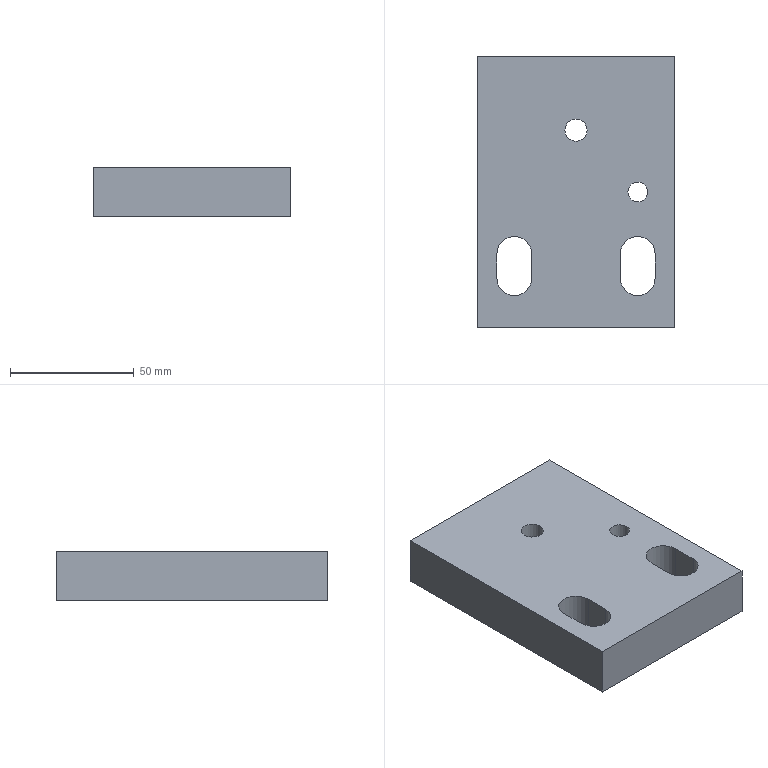Part | NX | features solid 2 | 1 solid | 18 faces | box 80 x 110 x 20 mm | volume 161289 mm3 | plane 11 | cylinder 7 | commonest cylinder face diameters 14 x4 8 x1 9 x1 13.5 x1
STEP:
#1=CARTESIAN_POINT('',(-1580.,335.,-55.));
#2=VERTEX_POINT('',#1);
#3=CARTESIAN_POINT('',(-1580.,445.,-55.));
#4=VERTEX_POINT('',#3);
#5=CARTESIAN_POINT('',(-1580.,375.,-55.));
#6=DIRECTION('',(0.,1.,0.));
#7=VECTOR('',#6,1000.);
#8=LINE('',#5,#7);
#9=EDGE_CURVE('',#2,#4,#8,.T.);
#10=ORIENTED_EDGE('',*,*,#9,.T.);
#11=CARTESIAN_POINT('',(-1500.,445.,-55.));
#12=VERTEX_POINT('',#11);
#13=CARTESIAN_POINT('',(-1580.,445.,-55.));
#14=DIRECTION('',(1.,0.,0.));
#15=VECTOR('',#14,1000.);
#16=LINE('',#13,#15);
#17=EDGE_CURVE('',#4,#12,#16,.T.);
#18=ORIENTED_EDGE('',*,*,#17,.T.);
#19=CARTESIAN_POINT('',(-1500.,335.,-55.));
#20=VERTEX_POINT('',#19);
#21=CARTESIAN_POINT('',(-1500.,475.,-55.));
#22=DIRECTION('',(0.,-1.,0.));
#23=VECTOR('',#22,1000.);
#24=LINE('',#21,#23);
#25=EDGE_CURVE('',#12,#20,#24,.T.);
#26=ORIENTED_EDGE('',*,*,#25,.T.);
#27=CARTESIAN_POINT('',(-1500.,335.,-55.));
#28=DIRECTION('',(-1.,0.,0.));
#29=VECTOR('',#28,1000.);
#30=LINE('',#27,#29);
#31=EDGE_CURVE('',#20,#2,#30,.T.);
#32=ORIENTED_EDGE('',*,*,#31,.T.);
#33=EDGE_LOOP('',(#10,#18,#26,#32));
#34=FACE_BOUND('',#33,.T.);
#35=CARTESIAN_POINT('',(-1572.,355.,-55.));
#36=VERTEX_POINT('',#35);
#37=CARTESIAN_POINT('',(-1572.,365.,-55.));
#38=VERTEX_POINT('',#37);
#39=CARTESIAN_POINT('',(-1572.,355.,-55.));
#40=DIRECTION('',(0.,1.,0.));
#41=VECTOR('',#40,1000.);
#42=LINE('',#39,#41);
#43=EDGE_CURVE('',#36,#38,#42,.T.);
#44=ORIENTED_EDGE('',*,*,#43,.F.);
#45=CARTESIAN_POINT('',(-1558.,355.,-55.));
#46=VERTEX_POINT('',#45);
#47=CARTESIAN_POINT('',(-1565.,355.,-55.));
#48=DIRECTION('',(0.,0.,1.));
#49=DIRECTION('',(1.,0.,0.));
#50=AXIS2_PLACEMENT_3D('',#47,#48,#49);
#51=CIRCLE('',#50,7.);
#52=EDGE_CURVE('',#36,#46,#51,.T.);
#53=ORIENTED_EDGE('',*,*,#52,.T.);
#54=CARTESIAN_POINT('',(-1558.,365.,-55.));
#55=VERTEX_POINT('',#54);
#56=CARTESIAN_POINT('',(-1558.,355.,-55.));
#57=DIRECTION('',(0.,1.,0.));
#58=VECTOR('',#57,1000.);
#59=LINE('',#56,#58);
#60=EDGE_CURVE('',#46,#55,#59,.T.);
#61=ORIENTED_EDGE('',*,*,#60,.T.);
#62=CARTESIAN_POINT('',(-1565.,365.,-55.));
#63=DIRECTION('',(0.,0.,1.));
#64=DIRECTION('',(1.,0.,0.));
#65=AXIS2_PLACEMENT_3D('',#62,#63,#64);
#66=CIRCLE('',#65,7.);
#67=EDGE_CURVE('',#55,#38,#66,.T.);
#68=ORIENTED_EDGE('',*,*,#67,.T.);
#69=EDGE_LOOP('',(#44,#53,#61,#68));
#70=FACE_BOUND('',#69,.T.);
#71=CARTESIAN_POINT('',(-1522.,355.,-55.));
#72=VERTEX_POINT('',#71);
#73=CARTESIAN_POINT('',(-1522.,365.,-55.));
#74=VERTEX_POINT('',#73);
#75=CARTESIAN_POINT('',(-1522.,355.,-55.));
#76=DIRECTION('',(0.,1.,0.));
#77=VECTOR('',#76,1000.);
#78=LINE('',#75,#77);
#79=EDGE_CURVE('',#72,#74,#78,.T.);
#80=ORIENTED_EDGE('',*,*,#79,.F.);
#81=CARTESIAN_POINT('',(-1508.,355.,-55.));
#82=VERTEX_POINT('',#81);
#83=CARTESIAN_POINT('',(-1515.,355.,-55.));
#84=DIRECTION('',(0.,0.,1.));
#85=DIRECTION('',(1.,0.,0.));
#86=AXIS2_PLACEMENT_3D('',#83,#84,#85);
#87=CIRCLE('',#86,7.);
#88=EDGE_CURVE('',#72,#82,#87,.T.);
#89=ORIENTED_EDGE('',*,*,#88,.T.);
#90=CARTESIAN_POINT('',(-1508.,365.,-55.));
#91=VERTEX_POINT('',#90);
#92=CARTESIAN_POINT('',(-1508.,355.,-55.));
#93=DIRECTION('',(0.,1.,0.));
#94=VECTOR('',#93,1000.);
#95=LINE('',#92,#94);
#96=EDGE_CURVE('',#82,#91,#95,.T.);
#97=ORIENTED_EDGE('',*,*,#96,.T.);
#98=CARTESIAN_POINT('',(-1515.,365.,-55.));
#99=DIRECTION('',(0.,0.,1.));
#100=DIRECTION('',(1.,0.,0.));
#101=AXIS2_PLACEMENT_3D('',#98,#99,#100);
#102=CIRCLE('',#101,7.);
#103=EDGE_CURVE('',#91,#74,#102,.T.);
#104=ORIENTED_EDGE('',*,*,#103,.T.);
#105=EDGE_LOOP('',(#80,#89,#97,#104));
#106=FACE_BOUND('',#105,.T.);
#107=CARTESIAN_POINT('',(-1533.25,415.,-55.));
#108=VERTEX_POINT('',#107);
#109=CARTESIAN_POINT('',(-1540.,415.,-55.));
#110=DIRECTION('',(0.,0.,1.));
#111=DIRECTION('',(1.,0.,0.));
#112=AXIS2_PLACEMENT_3D('',#109,#110,#111);
#113=CIRCLE('',#112,6.75);
#114=EDGE_CURVE('',#108,#108,#113,.T.);
#115=ORIENTED_EDGE('',*,*,#114,.T.);
#116=EDGE_LOOP('',(#115));
#117=FACE_BOUND('',#116,.T.);
#118=CARTESIAN_POINT('',(-1519.,390.,-55.));
#119=VERTEX_POINT('',#118);
#120=CARTESIAN_POINT('',(-1515.,390.,-55.));
#121=DIRECTION('',(0.,0.,-1.));
#122=DIRECTION('',(-1.,0.,0.));
#123=AXIS2_PLACEMENT_3D('',#120,#121,#122);
#124=CIRCLE('',#123,4.);
#125=EDGE_CURVE('',#119,#119,#124,.F.);
#126=ORIENTED_EDGE('',*,*,#125,.T.);
#127=EDGE_LOOP('',(#126));
#128=FACE_BOUND('',#127,.T.);
#129=CARTESIAN_POINT('',(-1580.,475.,-55.));
#130=DIRECTION('',(0.,0.,-1.));
#131=DIRECTION('',(-1.,0.,0.));
#132=AXIS2_PLACEMENT_3D('',#129,#130,#131);
#133=PLANE('',#132);
#134=ADVANCED_FACE('',(#34,#70,#106,#117,#128),#133,.T.);
#135=CARTESIAN_POINT('',(-1580.,335.,-35.));
#136=VERTEX_POINT('',#135);
#137=CARTESIAN_POINT('',(-1580.,445.,-35.));
#138=VERTEX_POINT('',#137);
#139=CARTESIAN_POINT('',(-1580.,375.,-35.));
#140=DIRECTION('',(0.,1.,0.));
#141=VECTOR('',#140,1000.);
#142=LINE('',#139,#141);
#143=EDGE_CURVE('',#136,#138,#142,.T.);
#144=ORIENTED_EDGE('',*,*,#143,.T.);
#145=CARTESIAN_POINT('',(-1580.,445.,-55.));
#146=DIRECTION('',(0.,0.,1.));
#147=VECTOR('',#146,1000.);
#148=LINE('',#145,#147);
#149=EDGE_CURVE('',#4,#138,#148,.T.);
#150=ORIENTED_EDGE('',*,*,#149,.F.);
#151=ORIENTED_EDGE('',*,*,#9,.F.);
#152=CARTESIAN_POINT('',(-1580.,335.,-55.));
#153=DIRECTION('',(0.,0.,1.));
#154=VECTOR('',#153,1000.);
#155=LINE('',#152,#154);
#156=EDGE_CURVE('',#2,#136,#155,.T.);
#157=ORIENTED_EDGE('',*,*,#156,.T.);
#158=EDGE_LOOP('',(#144,#150,#151,#157));
#159=FACE_BOUND('',#158,.T.);
#160=CARTESIAN_POINT('',(-1580.,375.,-55.));
#161=DIRECTION('',(1.,0.,0.));
#162=DIRECTION('',(0.,1.,0.));
#163=AXIS2_PLACEMENT_3D('',#160,#161,#162);
#164=PLANE('',#163);
#165=ADVANCED_FACE('',(#159),#164,.F.);
#166=CARTESIAN_POINT('',(-1500.,445.,-35.));
#167=VERTEX_POINT('',#166);
#168=CARTESIAN_POINT('',(-1580.,445.,-35.));
#169=DIRECTION('',(1.,0.,0.));
#170=VECTOR('',#169,1000.);
#171=LINE('',#168,#170);
#172=EDGE_CURVE('',#138,#167,#171,.T.);
#173=ORIENTED_EDGE('',*,*,#172,.T.);
#174=CARTESIAN_POINT('',(-1500.,445.,-55.));
#175=DIRECTION('',(0.,0.,1.));
#176=VECTOR('',#175,1000.);
#177=LINE('',#174,#176);
#178=EDGE_CURVE('',#12,#167,#177,.T.);
#179=ORIENTED_EDGE('',*,*,#178,.F.);
#180=ORIENTED_EDGE('',*,*,#17,.F.);
#181=ORIENTED_EDGE('',*,*,#149,.T.);
#182=EDGE_LOOP('',(#173,#179,#180,#181));
#183=FACE_BOUND('',#182,.T.);
#184=CARTESIAN_POINT('',(-1580.,445.,-55.));
#185=DIRECTION('',(0.,-1.,0.));
#186=DIRECTION('',(1.,0.,0.));
#187=AXIS2_PLACEMENT_3D('',#184,#185,#186);
#188=PLANE('',#187);
#189=ADVANCED_FACE('',(#183),#188,.F.);
#190=CARTESIAN_POINT('',(-1500.,335.,-35.));
#191=VERTEX_POINT('',#190);
#192=CARTESIAN_POINT('',(-1500.,475.,-35.));
#193=DIRECTION('',(0.,-1.,0.));
#194=VECTOR('',#193,1000.);
#195=LINE('',#192,#194);
#196=EDGE_CURVE('',#167,#191,#195,.T.);
#197=ORIENTED_EDGE('',*,*,#196,.T.);
#198=CARTESIAN_POINT('',(-1500.,335.,-55.));
#199=DIRECTION('',(0.,0.,1.));
#200=VECTOR('',#199,1000.);
#201=LINE('',#198,#200);
#202=EDGE_CURVE('',#20,#191,#201,.T.);
#203=ORIENTED_EDGE('',*,*,#202,.F.);
#204=ORIENTED_EDGE('',*,*,#25,.F.);
#205=ORIENTED_EDGE('',*,*,#178,.T.);
#206=EDGE_LOOP('',(#197,#203,#204,#205));
#207=FACE_BOUND('',#206,.T.);
#208=CARTESIAN_POINT('',(-1500.,475.,-55.));
#209=DIRECTION('',(-1.,0.,0.));
#210=DIRECTION('',(0.,0.,1.));
#211=AXIS2_PLACEMENT_3D('',#208,#209,#210);
#212=PLANE('',#211);
#213=ADVANCED_FACE('',(#207),#212,.F.);
#214=CARTESIAN_POINT('',(-1500.,335.,-35.));
#215=DIRECTION('',(-1.,0.,0.));
#216=VECTOR('',#215,1000.);
#217=LINE('',#214,#216);
#218=EDGE_CURVE('',#191,#136,#217,.T.);
#219=ORIENTED_EDGE('',*,*,#218,.T.);
#220=ORIENTED_EDGE('',*,*,#156,.F.);
#221=ORIENTED_EDGE('',*,*,#31,.F.);
#222=ORIENTED_EDGE('',*,*,#202,.T.);
#223=EDGE_LOOP('',(#219,#220,#221,#222));
#224=FACE_BOUND('',#223,.T.);
#225=CARTESIAN_POINT('',(-1500.,335.,-55.));
#226=DIRECTION('',(0.,1.,0.));
#227=DIRECTION('',(-1.,0.,0.));
#228=AXIS2_PLACEMENT_3D('',#225,#226,#227);
#229=PLANE('',#228);
#230=ADVANCED_FACE('',(#224),#229,.F.);
#231=CARTESIAN_POINT('',(-1519.,390.,-35.));
#232=VERTEX_POINT('',#231);
#233=CARTESIAN_POINT('',(-1515.,390.,-35.));
#234=DIRECTION('',(0.,0.,-1.));
#235=DIRECTION('',(-1.,0.,0.));
#236=AXIS2_PLACEMENT_3D('',#233,#234,#235);
#237=CIRCLE('',#236,4.);
#238=EDGE_CURVE('',#232,#232,#237,.T.);
#239=ORIENTED_EDGE('',*,*,#238,.T.);
#240=EDGE_LOOP('',(#239));
#241=FACE_BOUND('',#240,.T.);
#242=CARTESIAN_POINT('',(-1522.,355.,-35.));
#243=VERTEX_POINT('',#242);
#244=CARTESIAN_POINT('',(-1508.,355.,-35.));
#245=VERTEX_POINT('',#244);
#246=CARTESIAN_POINT('',(-1515.,355.,-35.));
#247=DIRECTION('',(0.,0.,1.));
#248=DIRECTION('',(1.,0.,0.));
#249=AXIS2_PLACEMENT_3D('',#246,#247,#248);
#250=CIRCLE('',#249,7.);
#251=EDGE_CURVE('',#243,#245,#250,.T.);
#252=ORIENTED_EDGE('',*,*,#251,.F.);
#253=CARTESIAN_POINT('',(-1522.,365.,-35.));
#254=VERTEX_POINT('',#253);
#255=CARTESIAN_POINT('',(-1522.,360.,-35.));
#256=DIRECTION('',(0.,1.,0.));
#257=VECTOR('',#256,1000.);
#258=LINE('',#255,#257);
#259=EDGE_CURVE('',#243,#254,#258,.T.);
#260=ORIENTED_EDGE('',*,*,#259,.T.);
#261=CARTESIAN_POINT('',(-1508.,365.,-35.));
#262=VERTEX_POINT('',#261);
#263=CARTESIAN_POINT('',(-1515.,365.,-35.));
#264=DIRECTION('',(0.,0.,1.));
#265=DIRECTION('',(1.,0.,0.));
#266=AXIS2_PLACEMENT_3D('',#263,#264,#265);
#267=CIRCLE('',#266,7.);
#268=EDGE_CURVE('',#262,#254,#267,.T.);
#269=ORIENTED_EDGE('',*,*,#268,.F.);
#270=CARTESIAN_POINT('',(-1508.,360.,-35.));
#271=DIRECTION('',(0.,1.,0.));
#272=VECTOR('',#271,1000.);
#273=LINE('',#270,#272);
#274=EDGE_CURVE('',#245,#262,#273,.T.);
#275=ORIENTED_EDGE('',*,*,#274,.F.);
#276=EDGE_LOOP('',(#252,#260,#269,#275));
#277=FACE_BOUND('',#276,.T.);
#278=CARTESIAN_POINT('',(-1572.,355.,-35.));
#279=VERTEX_POINT('',#278);
#280=CARTESIAN_POINT('',(-1558.,355.,-35.));
#281=VERTEX_POINT('',#280);
#282=CARTESIAN_POINT('',(-1565.,355.,-35.));
#283=DIRECTION('',(0.,0.,1.));
#284=DIRECTION('',(1.,0.,0.));
#285=AXIS2_PLACEMENT_3D('',#282,#283,#284);
#286=CIRCLE('',#285,7.);
#287=EDGE_CURVE('',#279,#281,#286,.T.);
#288=ORIENTED_EDGE('',*,*,#287,.F.);
#289=CARTESIAN_POINT('',(-1572.,365.,-35.));
#290=VERTEX_POINT('',#289);
#291=CARTESIAN_POINT('',(-1572.,360.,-35.));
#292=DIRECTION('',(0.,1.,0.));
#293=VECTOR('',#292,1000.);
#294=LINE('',#291,#293);
#295=EDGE_CURVE('',#279,#290,#294,.T.);
#296=ORIENTED_EDGE('',*,*,#295,.T.);
#297=CARTESIAN_POINT('',(-1558.,365.,-35.));
#298=VERTEX_POINT('',#297);
#299=CARTESIAN_POINT('',(-1565.,365.,-35.));
#300=DIRECTION('',(0.,0.,1.));
#301=DIRECTION('',(1.,0.,0.));
#302=AXIS2_PLACEMENT_3D('',#299,#300,#301);
#303=CIRCLE('',#302,7.);
#304=EDGE_CURVE('',#298,#290,#303,.T.);
#305=ORIENTED_EDGE('',*,*,#304,.F.);
#306=CARTESIAN_POINT('',(-1558.,360.,-35.));
#307=DIRECTION('',(0.,1.,0.));
#308=VECTOR('',#307,1000.);
#309=LINE('',#306,#308);
#310=EDGE_CURVE('',#281,#298,#309,.T.);
#311=ORIENTED_EDGE('',*,*,#310,.F.);
#312=EDGE_LOOP('',(#288,#296,#305,#311));
#313=FACE_BOUND('',#312,.T.);
#314=ORIENTED_EDGE('',*,*,#143,.F.);
#315=ORIENTED_EDGE('',*,*,#218,.F.);
#316=ORIENTED_EDGE('',*,*,#196,.F.);
#317=ORIENTED_EDGE('',*,*,#172,.F.);
#318=EDGE_LOOP('',(#314,#315,#316,#317));
#319=FACE_BOUND('',#318,.T.);
#320=CARTESIAN_POINT('',(-1544.5,415.,-35.));
#321=VERTEX_POINT('',#320);
#322=CARTESIAN_POINT('',(-1540.,415.,-35.));
#323=DIRECTION('',(0.,0.,-1.));
#324=DIRECTION('',(-1.,0.,0.));
#325=AXIS2_PLACEMENT_3D('',#322,#323,#324);
#326=CIRCLE('',#325,4.5);
#327=EDGE_CURVE('',#321,#321,#326,.F.);
#328=ORIENTED_EDGE('',*,*,#327,.F.);
#329=EDGE_LOOP('',(#328));
#330=FACE_BOUND('',#329,.T.);
#331=CARTESIAN_POINT('',(-1580.,475.,-35.));
#332=DIRECTION('',(0.,0.,-1.));
#333=DIRECTION('',(-1.,0.,0.));
#334=AXIS2_PLACEMENT_3D('',#331,#332,#333);
#335=PLANE('',#334);
#336=ADVANCED_FACE('',(#241,#277,#313,#319,#330),#335,.F.);
#337=ORIENTED_EDGE('',*,*,#295,.F.);
#338=CARTESIAN_POINT('',(-1572.,355.,-35.));
#339=DIRECTION('',(0.,0.,1.));
#340=VECTOR('',#339,1000.);
#341=LINE('',#338,#340);
#342=EDGE_CURVE('',#36,#279,#341,.T.);
#343=ORIENTED_EDGE('',*,*,#342,.F.);
#344=ORIENTED_EDGE('',*,*,#43,.T.);
#345=CARTESIAN_POINT('',(-1572.,365.,-35.));
#346=DIRECTION('',(0.,0.,1.));
#347=VECTOR('',#346,1000.);
#348=LINE('',#345,#347);
#349=EDGE_CURVE('',#38,#290,#348,.T.);
#350=ORIENTED_EDGE('',*,*,#349,.T.);
#351=EDGE_LOOP('',(#337,#343,#344,#350));
#352=FACE_BOUND('',#351,.T.);
#353=CARTESIAN_POINT('',(-1572.,360.,-35.));
#354=DIRECTION('',(-1.,0.,0.));
#355=DIRECTION('',(0.,0.,1.));
#356=AXIS2_PLACEMENT_3D('',#353,#354,#355);
#357=PLANE('',#356);
#358=ADVANCED_FACE('',(#352),#357,.F.);
#359=ORIENTED_EDGE('',*,*,#287,.T.);
#360=CARTESIAN_POINT('',(-1558.,355.,-35.));
#361=DIRECTION('',(0.,0.,1.));
#362=VECTOR('',#361,1000.);
#363=LINE('',#360,#362);
#364=EDGE_CURVE('',#46,#281,#363,.T.);
#365=ORIENTED_EDGE('',*,*,#364,.F.);
#366=ORIENTED_EDGE('',*,*,#52,.F.);
#367=ORIENTED_EDGE('',*,*,#342,.T.);
#368=EDGE_LOOP('',(#359,#365,#366,#367));
#369=FACE_BOUND('',#368,.T.);
#370=CARTESIAN_POINT('',(-1565.,355.,-35.));
#371=DIRECTION('',(0.,0.,1.));
#372=DIRECTION('',(1.,0.,0.));
#373=AXIS2_PLACEMENT_3D('',#370,#371,#372);
#374=CYLINDRICAL_SURFACE('',#373,7.);
#375=ADVANCED_FACE('',(#369),#374,.F.);
#376=ORIENTED_EDGE('',*,*,#310,.T.);
#377=CARTESIAN_POINT('',(-1558.,365.,-35.));
#378=DIRECTION('',(0.,0.,1.));
#379=VECTOR('',#378,1000.);
#380=LINE('',#377,#379);
#381=EDGE_CURVE('',#55,#298,#380,.T.);
#382=ORIENTED_EDGE('',*,*,#381,.F.);
#383=ORIENTED_EDGE('',*,*,#60,.F.);
#384=ORIENTED_EDGE('',*,*,#364,.T.);
#385=EDGE_LOOP('',(#376,#382,#383,#384));
#386=FACE_BOUND('',#385,.T.);
#387=CARTESIAN_POINT('',(-1558.,360.,-35.));
#388=DIRECTION('',(1.,0.,0.));
#389=DIRECTION('',(0.,0.,-1.));
#390=AXIS2_PLACEMENT_3D('',#387,#388,#389);
#391=PLANE('',#390);
#392=ADVANCED_FACE('',(#386),#391,.F.);
#393=ORIENTED_EDGE('',*,*,#304,.T.);
#394=ORIENTED_EDGE('',*,*,#349,.F.);
#395=ORIENTED_EDGE('',*,*,#67,.F.);
#396=ORIENTED_EDGE('',*,*,#381,.T.);
#397=EDGE_LOOP('',(#393,#394,#395,#396));
#398=FACE_BOUND('',#397,.T.);
#399=CARTESIAN_POINT('',(-1565.,365.,-35.));
#400=DIRECTION('',(0.,0.,1.));
#401=DIRECTION('',(1.,0.,0.));
#402=AXIS2_PLACEMENT_3D('',#399,#400,#401);
#403=CYLINDRICAL_SURFACE('',#402,7.);
#404=ADVANCED_FACE('',(#398),#403,.F.);
#405=ORIENTED_EDGE('',*,*,#259,.F.);
#406=CARTESIAN_POINT('',(-1522.,355.,-35.));
#407=DIRECTION('',(0.,0.,1.));
#408=VECTOR('',#407,1000.);
#409=LINE('',#406,#408);
#410=EDGE_CURVE('',#72,#243,#409,.T.);
#411=ORIENTED_EDGE('',*,*,#410,.F.);
#412=ORIENTED_EDGE('',*,*,#79,.T.);
#413=CARTESIAN_POINT('',(-1522.,365.,-35.));
#414=DIRECTION('',(0.,0.,1.));
#415=VECTOR('',#414,1000.);
#416=LINE('',#413,#415);
#417=EDGE_CURVE('',#74,#254,#416,.T.);
#418=ORIENTED_EDGE('',*,*,#417,.T.);
#419=EDGE_LOOP('',(#405,#411,#412,#418));
#420=FACE_BOUND('',#419,.T.);
#421=CARTESIAN_POINT('',(-1522.,360.,-35.));
#422=DIRECTION('',(-1.,0.,0.));
#423=DIRECTION('',(0.,0.,1.));
#424=AXIS2_PLACEMENT_3D('',#421,#422,#423);
#425=PLANE('',#424);
#426=ADVANCED_FACE('',(#420),#425,.F.);
#427=ORIENTED_EDGE('',*,*,#251,.T.);
#428=CARTESIAN_POINT('',(-1508.,355.,-35.));
#429=DIRECTION('',(0.,0.,1.));
#430=VECTOR('',#429,1000.);
#431=LINE('',#428,#430);
#432=EDGE_CURVE('',#82,#245,#431,.T.);
#433=ORIENTED_EDGE('',*,*,#432,.F.);
#434=ORIENTED_EDGE('',*,*,#88,.F.);
#435=ORIENTED_EDGE('',*,*,#410,.T.);
#436=EDGE_LOOP('',(#427,#433,#434,#435));
#437=FACE_BOUND('',#436,.T.);
#438=CARTESIAN_POINT('',(-1515.,355.,-35.));
#439=DIRECTION('',(0.,0.,1.));
#440=DIRECTION('',(1.,0.,0.));
#441=AXIS2_PLACEMENT_3D('',#438,#439,#440);
#442=CYLINDRICAL_SURFACE('',#441,7.);
#443=ADVANCED_FACE('',(#437),#442,.F.);
#444=ORIENTED_EDGE('',*,*,#274,.T.);
#445=CARTESIAN_POINT('',(-1508.,365.,-35.));
#446=DIRECTION('',(0.,0.,1.));
#447=VECTOR('',#446,1000.);
#448=LINE('',#445,#447);
#449=EDGE_CURVE('',#91,#262,#448,.T.);
#450=ORIENTED_EDGE('',*,*,#449,.F.);
#451=ORIENTED_EDGE('',*,*,#96,.F.);
#452=ORIENTED_EDGE('',*,*,#432,.T.);
#453=EDGE_LOOP('',(#444,#450,#451,#452));
#454=FACE_BOUND('',#453,.T.);
#455=CARTESIAN_POINT('',(-1508.,360.,-35.));
#456=DIRECTION('',(1.,0.,0.));
#457=DIRECTION('',(0.,0.,-1.));
#458=AXIS2_PLACEMENT_3D('',#455,#456,#457);
#459=PLANE('',#458);
#460=ADVANCED_FACE('',(#454),#459,.F.);
#461=ORIENTED_EDGE('',*,*,#268,.T.);
#462=ORIENTED_EDGE('',*,*,#417,.F.);
#463=ORIENTED_EDGE('',*,*,#103,.F.);
#464=ORIENTED_EDGE('',*,*,#449,.T.);
#465=EDGE_LOOP('',(#461,#462,#463,#464));
#466=FACE_BOUND('',#465,.T.);
#467=CARTESIAN_POINT('',(-1515.,365.,-35.));
#468=DIRECTION('',(0.,0.,1.));
#469=DIRECTION('',(1.,0.,0.));
#470=AXIS2_PLACEMENT_3D('',#467,#468,#469);
#471=CYLINDRICAL_SURFACE('',#470,7.);
#472=ADVANCED_FACE('',(#466),#471,.F.);
#473=ORIENTED_EDGE('',*,*,#238,.F.);
#474=EDGE_LOOP('',(#473));
#475=FACE_BOUND('',#474,.T.);
#476=ORIENTED_EDGE('',*,*,#125,.F.);
#477=EDGE_LOOP('',(#476));
#478=FACE_BOUND('',#477,.T.);
#479=CARTESIAN_POINT('',(-1515.,390.,-35.));
#480=DIRECTION('',(0.,0.,-1.));
#481=DIRECTION('',(-1.,0.,0.));
#482=AXIS2_PLACEMENT_3D('',#479,#480,#481);
#483=CYLINDRICAL_SURFACE('',#482,4.);
#484=ADVANCED_FACE('',(#475,#478),#483,.F.);
#485=ORIENTED_EDGE('',*,*,#327,.T.);
#486=EDGE_LOOP('',(#485));
#487=FACE_BOUND('',#486,.T.);
#488=CARTESIAN_POINT('',(-1535.5,415.,-46.5));
#489=VERTEX_POINT('',#488);
#490=CARTESIAN_POINT('',(-1540.,415.,-46.5));
#491=DIRECTION('',(0.,0.,1.));
#492=DIRECTION('',(1.,0.,0.));
#493=AXIS2_PLACEMENT_3D('',#490,#491,#492);
#494=CIRCLE('',#493,4.5);
#495=EDGE_CURVE('',#489,#489,#494,.T.);
#496=ORIENTED_EDGE('',*,*,#495,.F.);
#497=EDGE_LOOP('',(#496));
#498=FACE_BOUND('',#497,.T.);
#499=CARTESIAN_POINT('',(-1540.,415.,19.925));
#500=DIRECTION('',(0.,0.,1.));
#501=DIRECTION('',(1.,0.,0.));
#502=AXIS2_PLACEMENT_3D('',#499,#500,#501);
#503=CYLINDRICAL_SURFACE('',#502,4.5);
#504=ADVANCED_FACE('',(#487,#498),#503,.F.);
#505=ORIENTED_EDGE('',*,*,#495,.T.);
#506=EDGE_LOOP('',(#505));
#507=FACE_BOUND('',#506,.T.);
#508=CARTESIAN_POINT('',(-1533.25,415.,-46.5));
#509=VERTEX_POINT('',#508);
#510=CARTESIAN_POINT('',(-1540.,415.,-46.5));
#511=DIRECTION('',(0.,0.,1.));
#512=DIRECTION('',(1.,0.,0.));
#513=AXIS2_PLACEMENT_3D('',#510,#511,#512);
#514=CIRCLE('',#513,6.75);
#515=EDGE_CURVE('',#509,#509,#514,.T.);
#516=ORIENTED_EDGE('',*,*,#515,.F.);
#517=EDGE_LOOP('',(#516));
#518=FACE_BOUND('',#517,.T.);
#519=CARTESIAN_POINT('',(-1540.,415.,-46.5));
#520=DIRECTION('',(0.,0.,1.));
#521=DIRECTION('',(1.,0.,0.));
#522=AXIS2_PLACEMENT_3D('',#519,#520,#521);
#523=PLANE('',#522);
#524=ADVANCED_FACE('',(#507,#518),#523,.F.);
#525=ORIENTED_EDGE('',*,*,#515,.T.);
#526=EDGE_LOOP('',(#525));
#527=FACE_BOUND('',#526,.T.);
#528=ORIENTED_EDGE('',*,*,#114,.F.);
#529=EDGE_LOOP('',(#528));
#530=FACE_BOUND('',#529,.T.);
#531=CARTESIAN_POINT('',(-1540.,415.,-55.));
#532=DIRECTION('',(0.,0.,1.));
#533=DIRECTION('',(1.,0.,0.));
#534=AXIS2_PLACEMENT_3D('',#531,#532,#533);
#535=CYLINDRICAL_SURFACE('',#534,6.75);
#536=ADVANCED_FACE('',(#527,#530),#535,.F.);
#537=CLOSED_SHELL('',(#134,#165,#189,#213,#230,#336,#358,#375,#392,#404,#426,#443,#460,#472,#484,#504,#524,#536));
#538=MANIFOLD_SOLID_BREP('',#537);
#539=(LENGTH_UNIT()NAMED_UNIT(*)SI_UNIT(.MILLI.,.METRE.));
#540=UNCERTAINTY_MEASURE_WITH_UNIT(LENGTH_MEASURE(0.00001),#539,'','');
#541=(NAMED_UNIT(*)PLANE_ANGLE_UNIT()SI_UNIT($,.RADIAN.));
#542=(NAMED_UNIT(*)SI_UNIT($,.STERADIAN.)SOLID_ANGLE_UNIT());
#543=(GEOMETRIC_REPRESENTATION_CONTEXT(3)GLOBAL_UNCERTAINTY_ASSIGNED_CONTEXT((#540))GLOBAL_UNIT_ASSIGNED_CONTEXT((#539,#541,#542))REPRESENTATION_CONTEXT('',''));
#544=ADVANCED_BREP_SHAPE_REPRESENTATION('',(#538),#543);